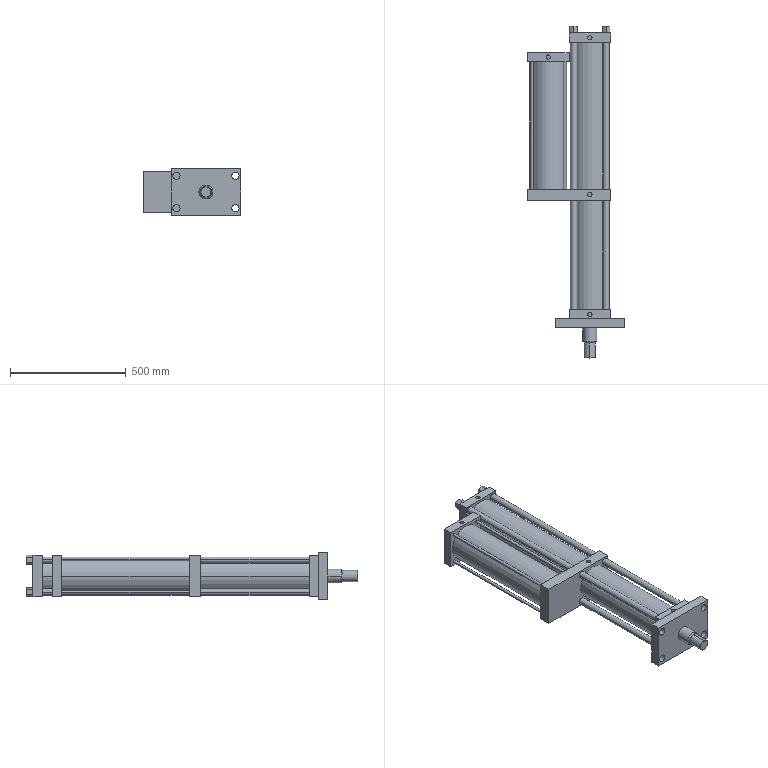Part | SolidWorks | features BaseBody 1, ICE 1, MoveCopyBody 1, MoveFace 1 | 2 solids | 124 faces | box 420 x 1435 x 200 mm | volume 41260242 mm3 | plane 68 | cylinder 52 | cone 4 | commonest cylinder face diameters 28 x16 12 x8 18.5 x8 32 x8 160 x4 48 x2